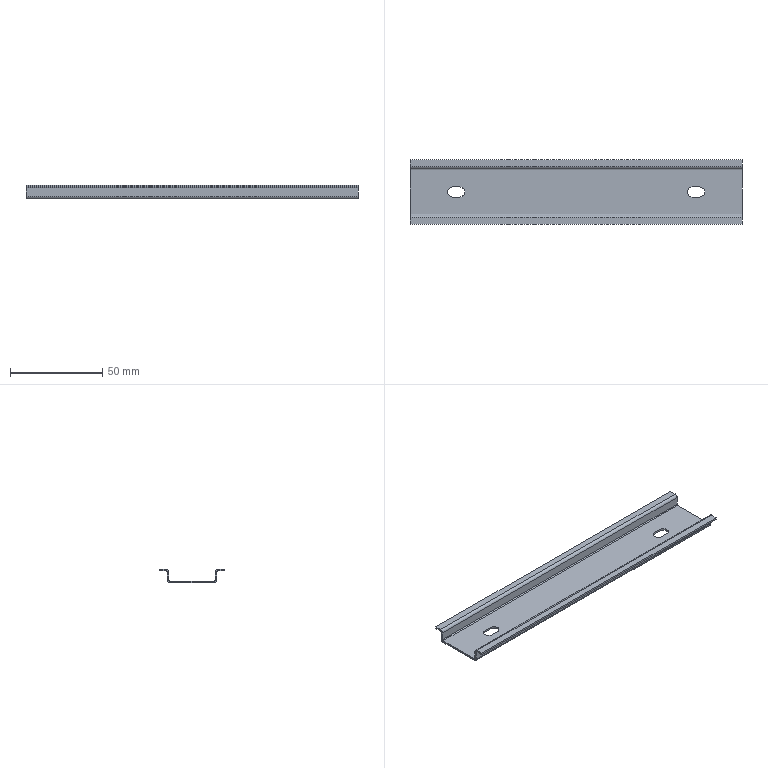Part | SolidWorks | features BaseBody 1 | 1 solid | 48 faces | box 180 x 35 x 7.5 mm | volume 8239 mm3 | plane 34 | cylinder 14 | commonest cylinder face diameters 5.5 x6 1 x4 3 x4
STEP:
#1=CARTESIAN_POINT('',(-67.,-2.75,0.));
#2=VERTEX_POINT('',#1);
#3=CARTESIAN_POINT('',(-63.,-2.75,0.));
#4=VERTEX_POINT('',#3);
#5=CARTESIAN_POINT('',(-67.,-2.75,0.));
#6=DIRECTION('',(1.,0.,0.));
#7=VECTOR('',#6,1000.);
#8=LINE('',#5,#7);
#9=EDGE_CURVE('',#2,#4,#8,.T.);
#10=ORIENTED_EDGE('',*,*,#9,.T.);
#11=CARTESIAN_POINT('',(-63.,-2.75,-1.));
#12=VERTEX_POINT('',#11);
#13=CARTESIAN_POINT('',(-63.,-2.75,-1.));
#14=DIRECTION('',(0.,0.,1.));
#15=VECTOR('',#14,1000.);
#16=LINE('',#13,#15);
#17=EDGE_CURVE('',#12,#4,#16,.T.);
#18=ORIENTED_EDGE('',*,*,#17,.F.);
#19=CARTESIAN_POINT('',(-67.,-2.75,-1.));
#20=VERTEX_POINT('',#19);
#21=CARTESIAN_POINT('',(-67.,-2.75,-1.));
#22=DIRECTION('',(1.,0.,0.));
#23=VECTOR('',#22,1000.);
#24=LINE('',#21,#23);
#25=EDGE_CURVE('',#20,#12,#24,.T.);
#26=ORIENTED_EDGE('',*,*,#25,.F.);
#27=CARTESIAN_POINT('',(-67.,-2.75,-1.));
#28=DIRECTION('',(0.,0.,1.));
#29=VECTOR('',#28,1000.);
#30=LINE('',#27,#29);
#31=EDGE_CURVE('',#20,#2,#30,.T.);
#32=ORIENTED_EDGE('',*,*,#31,.T.);
#33=EDGE_LOOP('',(#10,#18,#26,#32));
#34=FACE_OUTER_BOUND('',#33,.T.);
#35=CARTESIAN_POINT('',(-67.,-2.75,-1.));
#36=DIRECTION('',(0.,-1.,0.));
#37=DIRECTION('',(-1.,0.,0.));
#38=AXIS2_PLACEMENT_3D('',#35,#36,#37);
#39=PLANE('',#38);
#40=ADVANCED_FACE('',(#34),#39,.F.);
#41=CARTESIAN_POINT('',(-60.25,0.,-1.));
#42=VERTEX_POINT('',#41);
#43=CARTESIAN_POINT('',(-60.25,0.,0.));
#44=VERTEX_POINT('',#43);
#45=CARTESIAN_POINT('',(-60.25,0.,-1.));
#46=DIRECTION('',(0.,0.,1.));
#47=VECTOR('',#46,1000.);
#48=LINE('',#45,#47);
#49=EDGE_CURVE('',#42,#44,#48,.T.);
#50=ORIENTED_EDGE('',*,*,#49,.F.);
#51=CARTESIAN_POINT('',(-63.,0.,-1.));
#52=DIRECTION('',(0.,0.,1.));
#53=DIRECTION('',(1.,0.,0.));
#54=AXIS2_PLACEMENT_3D('',#51,#52,#53);
#55=CIRCLE('',#54,2.75);
#56=EDGE_CURVE('',#12,#42,#55,.T.);
#57=ORIENTED_EDGE('',*,*,#56,.F.);
#58=ORIENTED_EDGE('',*,*,#17,.T.);
#59=CARTESIAN_POINT('',(-63.,0.,0.));
#60=DIRECTION('',(0.,0.,1.));
#61=DIRECTION('',(1.,0.,0.));
#62=AXIS2_PLACEMENT_3D('',#59,#60,#61);
#63=CIRCLE('',#62,2.75);
#64=EDGE_CURVE('',#4,#44,#63,.T.);
#65=ORIENTED_EDGE('',*,*,#64,.T.);
#66=EDGE_LOOP('',(#50,#57,#58,#65));
#67=FACE_OUTER_BOUND('',#66,.T.);
#68=CARTESIAN_POINT('',(-63.,0.,-1.));
#69=DIRECTION('',(0.,0.,1.));
#70=DIRECTION('',(1.,0.,0.));
#71=AXIS2_PLACEMENT_3D('',#68,#69,#70);
#72=CYLINDRICAL_SURFACE('',#71,2.75);
#73=ADVANCED_FACE('',(#67),#72,.F.);
#74=CARTESIAN_POINT('',(-63.,2.75,0.));
#75=VERTEX_POINT('',#74);
#76=CARTESIAN_POINT('',(-67.,2.75,0.));
#77=VERTEX_POINT('',#76);
#78=CARTESIAN_POINT('',(-67.,2.75,0.));
#79=DIRECTION('',(-1.,0.,0.));
#80=VECTOR('',#79,1000.);
#81=LINE('',#78,#80);
#82=EDGE_CURVE('',#75,#77,#81,.T.);
#83=ORIENTED_EDGE('',*,*,#82,.T.);
#84=CARTESIAN_POINT('',(-67.,2.75,-1.));
#85=VERTEX_POINT('',#84);
#86=CARTESIAN_POINT('',(-67.,2.75,-1.));
#87=DIRECTION('',(0.,0.,1.));
#88=VECTOR('',#87,1000.);
#89=LINE('',#86,#88);
#90=EDGE_CURVE('',#85,#77,#89,.T.);
#91=ORIENTED_EDGE('',*,*,#90,.F.);
#92=CARTESIAN_POINT('',(-63.,2.75,-1.));
#93=VERTEX_POINT('',#92);
#94=CARTESIAN_POINT('',(-67.,2.75,-1.));
#95=DIRECTION('',(-1.,0.,0.));
#96=VECTOR('',#95,1000.);
#97=LINE('',#94,#96);
#98=EDGE_CURVE('',#93,#85,#97,.T.);
#99=ORIENTED_EDGE('',*,*,#98,.F.);
#100=CARTESIAN_POINT('',(-63.,2.75,-1.));
#101=DIRECTION('',(0.,0.,1.));
#102=VECTOR('',#101,1000.);
#103=LINE('',#100,#102);
#104=EDGE_CURVE('',#93,#75,#103,.T.);
#105=ORIENTED_EDGE('',*,*,#104,.T.);
#106=EDGE_LOOP('',(#83,#91,#99,#105));
#107=FACE_OUTER_BOUND('',#106,.T.);
#108=CARTESIAN_POINT('',(-67.,2.75,-1.));
#109=DIRECTION('',(0.,1.,0.));
#110=DIRECTION('',(1.,0.,0.));
#111=AXIS2_PLACEMENT_3D('',#108,#109,#110);
#112=PLANE('',#111);
#113=ADVANCED_FACE('',(#107),#112,.F.);
#114=CARTESIAN_POINT('',(-67.,0.,0.));
#115=DIRECTION('',(0.,0.,1.));
#116=DIRECTION('',(1.,0.,0.));
#117=AXIS2_PLACEMENT_3D('',#114,#115,#116);
#118=CIRCLE('',#117,2.75);
#119=EDGE_CURVE('',#77,#2,#118,.T.);
#120=ORIENTED_EDGE('',*,*,#119,.T.);
#121=ORIENTED_EDGE('',*,*,#31,.F.);
#122=CARTESIAN_POINT('',(-67.,0.,-1.));
#123=DIRECTION('',(0.,0.,1.));
#124=DIRECTION('',(1.,0.,0.));
#125=AXIS2_PLACEMENT_3D('',#122,#123,#124);
#126=CIRCLE('',#125,2.75);
#127=EDGE_CURVE('',#85,#20,#126,.T.);
#128=ORIENTED_EDGE('',*,*,#127,.F.);
#129=ORIENTED_EDGE('',*,*,#90,.T.);
#130=EDGE_LOOP('',(#120,#121,#128,#129));
#131=FACE_OUTER_BOUND('',#130,.T.);
#132=CARTESIAN_POINT('',(-67.,0.,-1.));
#133=DIRECTION('',(0.,0.,1.));
#134=DIRECTION('',(1.,0.,0.));
#135=AXIS2_PLACEMENT_3D('',#132,#133,#134);
#136=CYLINDRICAL_SURFACE('',#135,2.75);
#137=ADVANCED_FACE('',(#131),#136,.F.);
#138=CARTESIAN_POINT('',(67.,2.75,0.));
#139=VERTEX_POINT('',#138);
#140=CARTESIAN_POINT('',(63.,2.75,0.));
#141=VERTEX_POINT('',#140);
#142=CARTESIAN_POINT('',(67.,2.75,0.));
#143=DIRECTION('',(-1.,0.,0.));
#144=VECTOR('',#143,1000.);
#145=LINE('',#142,#144);
#146=EDGE_CURVE('',#139,#141,#145,.T.);
#147=ORIENTED_EDGE('',*,*,#146,.T.);
#148=CARTESIAN_POINT('',(63.,2.75,-1.));
#149=VERTEX_POINT('',#148);
#150=CARTESIAN_POINT('',(63.,2.75,-1.));
#151=DIRECTION('',(0.,0.,1.));
#152=VECTOR('',#151,1000.);
#153=LINE('',#150,#152);
#154=EDGE_CURVE('',#149,#141,#153,.T.);
#155=ORIENTED_EDGE('',*,*,#154,.F.);
#156=CARTESIAN_POINT('',(67.,2.75,-1.));
#157=VERTEX_POINT('',#156);
#158=CARTESIAN_POINT('',(67.,2.75,-1.));
#159=DIRECTION('',(-1.,0.,0.));
#160=VECTOR('',#159,1000.);
#161=LINE('',#158,#160);
#162=EDGE_CURVE('',#157,#149,#161,.T.);
#163=ORIENTED_EDGE('',*,*,#162,.F.);
#164=CARTESIAN_POINT('',(67.,2.75,-1.));
#165=DIRECTION('',(0.,0.,1.));
#166=VECTOR('',#165,1000.);
#167=LINE('',#164,#166);
#168=EDGE_CURVE('',#157,#139,#167,.T.);
#169=ORIENTED_EDGE('',*,*,#168,.T.);
#170=EDGE_LOOP('',(#147,#155,#163,#169));
#171=FACE_OUTER_BOUND('',#170,.T.);
#172=CARTESIAN_POINT('',(67.,2.75,-1.));
#173=DIRECTION('',(0.,1.,0.));
#174=DIRECTION('',(1.,0.,0.));
#175=AXIS2_PLACEMENT_3D('',#172,#173,#174);
#176=PLANE('',#175);
#177=ADVANCED_FACE('',(#171),#176,.F.);
#178=CARTESIAN_POINT('',(63.,-2.75,0.));
#179=VERTEX_POINT('',#178);
#180=CARTESIAN_POINT('',(63.,0.,0.));
#181=DIRECTION('',(0.,0.,1.));
#182=DIRECTION('',(-1.,0.,0.));
#183=AXIS2_PLACEMENT_3D('',#180,#181,#182);
#184=CIRCLE('',#183,2.75);
#185=EDGE_CURVE('',#141,#179,#184,.T.);
#186=ORIENTED_EDGE('',*,*,#185,.T.);
#187=CARTESIAN_POINT('',(63.,-2.75,-1.));
#188=VERTEX_POINT('',#187);
#189=CARTESIAN_POINT('',(63.,-2.75,-1.));
#190=DIRECTION('',(0.,0.,1.));
#191=VECTOR('',#190,1000.);
#192=LINE('',#189,#191);
#193=EDGE_CURVE('',#188,#179,#192,.T.);
#194=ORIENTED_EDGE('',*,*,#193,.F.);
#195=CARTESIAN_POINT('',(63.,0.,-1.));
#196=DIRECTION('',(0.,0.,1.));
#197=DIRECTION('',(-1.,0.,0.));
#198=AXIS2_PLACEMENT_3D('',#195,#196,#197);
#199=CIRCLE('',#198,2.75);
#200=EDGE_CURVE('',#149,#188,#199,.T.);
#201=ORIENTED_EDGE('',*,*,#200,.F.);
#202=ORIENTED_EDGE('',*,*,#154,.T.);
#203=EDGE_LOOP('',(#186,#194,#201,#202));
#204=FACE_OUTER_BOUND('',#203,.T.);
#205=CARTESIAN_POINT('',(63.,0.,-1.));
#206=DIRECTION('',(0.,0.,1.));
#207=DIRECTION('',(1.,0.,0.));
#208=AXIS2_PLACEMENT_3D('',#205,#206,#207);
#209=CYLINDRICAL_SURFACE('',#208,2.75);
#210=ADVANCED_FACE('',(#204),#209,.F.);
#211=CARTESIAN_POINT('',(67.,-2.75,0.));
#212=VERTEX_POINT('',#211);
#213=CARTESIAN_POINT('',(67.,-2.75,0.));
#214=DIRECTION('',(1.,0.,0.));
#215=VECTOR('',#214,1000.);
#216=LINE('',#213,#215);
#217=EDGE_CURVE('',#179,#212,#216,.T.);
#218=ORIENTED_EDGE('',*,*,#217,.T.);
#219=CARTESIAN_POINT('',(67.,-2.75,-1.));
#220=VERTEX_POINT('',#219);
#221=CARTESIAN_POINT('',(67.,-2.75,-1.));
#222=DIRECTION('',(0.,0.,1.));
#223=VECTOR('',#222,1000.);
#224=LINE('',#221,#223);
#225=EDGE_CURVE('',#220,#212,#224,.T.);
#226=ORIENTED_EDGE('',*,*,#225,.F.);
#227=CARTESIAN_POINT('',(67.,-2.75,-1.));
#228=DIRECTION('',(1.,0.,0.));
#229=VECTOR('',#228,1000.);
#230=LINE('',#227,#229);
#231=EDGE_CURVE('',#188,#220,#230,.T.);
#232=ORIENTED_EDGE('',*,*,#231,.F.);
#233=ORIENTED_EDGE('',*,*,#193,.T.);
#234=EDGE_LOOP('',(#218,#226,#232,#233));
#235=FACE_OUTER_BOUND('',#234,.T.);
#236=CARTESIAN_POINT('',(67.,-2.75,-1.));
#237=DIRECTION('',(0.,-1.,0.));
#238=DIRECTION('',(0.,0.,-1.));
#239=AXIS2_PLACEMENT_3D('',#236,#237,#238);
#240=PLANE('',#239);
#241=ADVANCED_FACE('',(#235),#240,.F.);
#242=CARTESIAN_POINT('',(69.75,0.,-1.));
#243=VERTEX_POINT('',#242);
#244=CARTESIAN_POINT('',(69.75,0.,0.));
#245=VERTEX_POINT('',#244);
#246=CARTESIAN_POINT('',(69.75,0.,-1.));
#247=DIRECTION('',(0.,0.,1.));
#248=VECTOR('',#247,1000.);
#249=LINE('',#246,#248);
#250=EDGE_CURVE('',#243,#245,#249,.T.);
#251=ORIENTED_EDGE('',*,*,#250,.F.);
#252=CARTESIAN_POINT('',(67.,0.,-1.));
#253=DIRECTION('',(0.,0.,1.));
#254=DIRECTION('',(-1.,0.,0.));
#255=AXIS2_PLACEMENT_3D('',#252,#253,#254);
#256=CIRCLE('',#255,2.75);
#257=EDGE_CURVE('',#220,#243,#256,.T.);
#258=ORIENTED_EDGE('',*,*,#257,.F.);
#259=ORIENTED_EDGE('',*,*,#225,.T.);
#260=CARTESIAN_POINT('',(67.,0.,0.));
#261=DIRECTION('',(0.,0.,1.));
#262=DIRECTION('',(-1.,0.,0.));
#263=AXIS2_PLACEMENT_3D('',#260,#261,#262);
#264=CIRCLE('',#263,2.75);
#265=EDGE_CURVE('',#212,#245,#264,.T.);
#266=ORIENTED_EDGE('',*,*,#265,.T.);
#267=EDGE_LOOP('',(#251,#258,#259,#266));
#268=FACE_OUTER_BOUND('',#267,.T.);
#269=CARTESIAN_POINT('',(67.,0.,-1.));
#270=DIRECTION('',(0.,0.,1.));
#271=DIRECTION('',(1.,0.,0.));
#272=AXIS2_PLACEMENT_3D('',#269,#270,#271);
#273=CYLINDRICAL_SURFACE('',#272,2.75);
#274=ADVANCED_FACE('',(#268),#273,.F.);
#275=CARTESIAN_POINT('',(-90.,-17.5,5.5));
#276=VERTEX_POINT('',#275);
#277=CARTESIAN_POINT('',(90.,-17.5,5.5));
#278=VERTEX_POINT('',#277);
#279=CARTESIAN_POINT('',(90.,-17.5,5.5));
#280=DIRECTION('',(1.,0.,0.));
#281=VECTOR('',#280,1000.);
#282=LINE('',#279,#281);
#283=EDGE_CURVE('',#276,#278,#282,.T.);
#284=ORIENTED_EDGE('',*,*,#283,.T.);
#285=CARTESIAN_POINT('',(90.,-17.5,6.5));
#286=VERTEX_POINT('',#285);
#287=CARTESIAN_POINT('',(90.,-17.5,6.5));
#288=DIRECTION('',(0.,0.,-1.));
#289=VECTOR('',#288,1000.);
#290=LINE('',#287,#289);
#291=EDGE_CURVE('',#286,#278,#290,.T.);
#292=ORIENTED_EDGE('',*,*,#291,.F.);
#293=CARTESIAN_POINT('',(-90.,-17.5,6.5));
#294=VERTEX_POINT('',#293);
#295=CARTESIAN_POINT('',(0.,-17.5,6.5));
#296=DIRECTION('',(1.,0.,0.));
#297=VECTOR('',#296,1000.);
#298=LINE('',#295,#297);
#299=EDGE_CURVE('',#294,#286,#298,.T.);
#300=ORIENTED_EDGE('',*,*,#299,.F.);
#301=CARTESIAN_POINT('',(-90.,-17.5,6.5));
#302=DIRECTION('',(0.,0.,-1.));
#303=VECTOR('',#302,1000.);
#304=LINE('',#301,#303);
#305=EDGE_CURVE('',#294,#276,#304,.T.);
#306=ORIENTED_EDGE('',*,*,#305,.T.);
#307=EDGE_LOOP('',(#284,#292,#300,#306));
#308=FACE_OUTER_BOUND('',#307,.T.);
#309=CARTESIAN_POINT('',(90.,-17.5,6.5));
#310=DIRECTION('',(0.,1.,0.));
#311=DIRECTION('',(0.,0.,-1.));
#312=AXIS2_PLACEMENT_3D('',#309,#310,#311);
#313=PLANE('',#312);
#314=ADVANCED_FACE('',(#308),#313,.F.);
#315=CARTESIAN_POINT('',(-90.,-14.,5.5));
#316=VERTEX_POINT('',#315);
#317=CARTESIAN_POINT('',(-90.,-17.5,5.5));
#318=DIRECTION('',(0.,-1.,0.));
#319=VECTOR('',#318,1000.);
#320=LINE('',#317,#319);
#321=EDGE_CURVE('',#316,#276,#320,.T.);
#322=ORIENTED_EDGE('',*,*,#321,.F.);
#323=CARTESIAN_POINT('',(90.,-14.,5.5));
#324=VERTEX_POINT('',#323);
#325=CARTESIAN_POINT('',(90.,-14.,5.5));
#326=DIRECTION('',(-1.,0.,0.));
#327=VECTOR('',#326,1000.);
#328=LINE('',#325,#327);
#329=EDGE_CURVE('',#324,#316,#328,.T.);
#330=ORIENTED_EDGE('',*,*,#329,.F.);
#331=CARTESIAN_POINT('',(90.,-13.5,5.5));
#332=DIRECTION('',(0.,1.,0.));
#333=VECTOR('',#332,1000.);
#334=LINE('',#331,#333);
#335=EDGE_CURVE('',#278,#324,#334,.T.);
#336=ORIENTED_EDGE('',*,*,#335,.F.);
#337=ORIENTED_EDGE('',*,*,#283,.F.);
#338=EDGE_LOOP('',(#322,#330,#336,#337));
#339=FACE_OUTER_BOUND('',#338,.T.);
#340=CARTESIAN_POINT('',(0.,0.,5.5));
#341=DIRECTION('',(0.,0.,-1.));
#342=DIRECTION('',(-1.,0.,0.));
#343=AXIS2_PLACEMENT_3D('',#340,#341,#342);
#344=PLANE('',#343);
#345=ADVANCED_FACE('',(#339),#344,.T.);
#346=CARTESIAN_POINT('',(-90.,-14.,6.5));
#347=VERTEX_POINT('',#346);
#348=CARTESIAN_POINT('',(90.,-14.,6.5));
#349=VERTEX_POINT('',#348);
#350=CARTESIAN_POINT('',(90.,-14.,6.5));
#351=DIRECTION('',(1.,0.,0.));
#352=VECTOR('',#351,1000.);
#353=LINE('',#350,#352);
#354=EDGE_CURVE('',#347,#349,#353,.T.);
#355=ORIENTED_EDGE('',*,*,#354,.F.);
#356=CARTESIAN_POINT('',(-90.,0.,6.5));
#357=DIRECTION('',(0.,-1.,0.));
#358=VECTOR('',#357,1000.);
#359=LINE('',#356,#358);
#360=EDGE_CURVE('',#347,#294,#359,.T.);
#361=ORIENTED_EDGE('',*,*,#360,.T.);
#362=ORIENTED_EDGE('',*,*,#299,.T.);
#363=CARTESIAN_POINT('',(90.,0.,6.5));
#364=DIRECTION('',(0.,1.,0.));
#365=VECTOR('',#364,1000.);
#366=LINE('',#363,#365);
#367=EDGE_CURVE('',#286,#349,#366,.T.);
#368=ORIENTED_EDGE('',*,*,#367,.T.);
#369=EDGE_LOOP('',(#355,#361,#362,#368));
#370=FACE_OUTER_BOUND('',#369,.T.);
#371=CARTESIAN_POINT('',(0.,0.,6.5));
#372=DIRECTION('',(0.,0.,-1.));
#373=DIRECTION('',(-1.,0.,0.));
#374=AXIS2_PLACEMENT_3D('',#371,#372,#373);
#375=PLANE('',#374);
#376=ADVANCED_FACE('',(#370),#375,.F.);
#377=CARTESIAN_POINT('',(-90.,-14.,5.5));
#378=DIRECTION('',(0.,0.,1.));
#379=VECTOR('',#378,1000.);
#380=LINE('',#377,#379);
#381=EDGE_CURVE('',#316,#347,#380,.T.);
#382=ORIENTED_EDGE('',*,*,#381,.F.);
#383=ORIENTED_EDGE('',*,*,#321,.T.);
#384=ORIENTED_EDGE('',*,*,#305,.F.);
#385=ORIENTED_EDGE('',*,*,#360,.F.);
#386=EDGE_LOOP('',(#382,#383,#384,#385));
#387=FACE_OUTER_BOUND('',#386,.T.);
#388=CARTESIAN_POINT('',(-90.,-17.5,6.5));
#389=DIRECTION('',(1.,0.,0.));
#390=DIRECTION('',(0.,0.,-1.));
#391=AXIS2_PLACEMENT_3D('',#388,#389,#390);
#392=PLANE('',#391);
#393=ADVANCED_FACE('',(#387),#392,.F.);
#394=CARTESIAN_POINT('',(90.,-14.,6.5));
#395=DIRECTION('',(0.,0.,1.));
#396=VECTOR('',#395,1000.);
#397=LINE('',#394,#396);
#398=EDGE_CURVE('',#324,#349,#397,.T.);
#399=ORIENTED_EDGE('',*,*,#398,.T.);
#400=ORIENTED_EDGE('',*,*,#367,.F.);
#401=ORIENTED_EDGE('',*,*,#291,.T.);
#402=ORIENTED_EDGE('',*,*,#335,.T.);
#403=EDGE_LOOP('',(#399,#400,#401,#402));
#404=FACE_OUTER_BOUND('',#403,.T.);
#405=CARTESIAN_POINT('',(90.,-13.5,6.5));
#406=DIRECTION('',(-1.,0.,0.));
#407=DIRECTION('',(0.,1.,0.));
#408=AXIS2_PLACEMENT_3D('',#405,#406,#407);
#409=PLANE('',#408);
#410=ADVANCED_FACE('',(#404),#409,.F.);
#411=CARTESIAN_POINT('',(-90.,-13.5,5.));
#412=VERTEX_POINT('',#411);
#413=CARTESIAN_POINT('',(90.,-13.5,5.));
#414=VERTEX_POINT('',#413);
#415=CARTESIAN_POINT('',(-90.,-13.5,5.));
#416=DIRECTION('',(1.,0.,0.));
#417=VECTOR('',#416,1000.);
#418=LINE('',#415,#417);
#419=EDGE_CURVE('',#412,#414,#418,.T.);
#420=ORIENTED_EDGE('',*,*,#419,.T.);
#421=CARTESIAN_POINT('',(90.,-14.,5.));
#422=DIRECTION('',(1.,0.,0.));
#423=DIRECTION('',(0.,0.,1.));
#424=AXIS2_PLACEMENT_3D('',#421,#422,#423);
#425=CIRCLE('',#424,0.5);
#426=EDGE_CURVE('',#414,#324,#425,.T.);
#427=ORIENTED_EDGE('',*,*,#426,.T.);
#428=ORIENTED_EDGE('',*,*,#329,.T.);
#429=CARTESIAN_POINT('',(-90.,-14.,5.));
#430=DIRECTION('',(-1.,0.,0.));
#431=DIRECTION('',(0.,0.,1.));
#432=AXIS2_PLACEMENT_3D('',#429,#430,#431);
#433=CIRCLE('',#432,0.5);
#434=EDGE_CURVE('',#316,#412,#433,.T.);
#435=ORIENTED_EDGE('',*,*,#434,.T.);
#436=EDGE_LOOP('',(#420,#427,#428,#435));
#437=FACE_OUTER_BOUND('',#436,.T.);
#438=CARTESIAN_POINT('',(-90.,-14.,5.));
#439=DIRECTION('',(-1.,0.,0.));
#440=DIRECTION('',(0.,0.,1.));
#441=AXIS2_PLACEMENT_3D('',#438,#439,#440);
#442=CYLINDRICAL_SURFACE('',#441,0.5);
#443=ADVANCED_FACE('',(#437),#442,.F.);
#444=CARTESIAN_POINT('',(-90.,-12.5,5.));
#445=VERTEX_POINT('',#444);
#446=CARTESIAN_POINT('',(90.,-12.5,5.));
#447=VERTEX_POINT('',#446);
#448=CARTESIAN_POINT('',(-90.,-12.5,5.));
#449=DIRECTION('',(1.,0.,0.));
#450=VECTOR('',#449,1000.);
#451=LINE('',#448,#450);
#452=EDGE_CURVE('',#445,#447,#451,.T.);
#453=ORIENTED_EDGE('',*,*,#452,.F.);
#454=CARTESIAN_POINT('',(-90.,-14.,5.));
#455=DIRECTION('',(-1.,0.,0.));
#456=DIRECTION('',(0.,0.,1.));
#457=AXIS2_PLACEMENT_3D('',#454,#455,#456);
#458=CIRCLE('',#457,1.5);
#459=EDGE_CURVE('',#347,#445,#458,.T.);
#460=ORIENTED_EDGE('',*,*,#459,.F.);
#461=ORIENTED_EDGE('',*,*,#354,.T.);
#462=CARTESIAN_POINT('',(90.,-14.,5.));
#463=DIRECTION('',(1.,0.,0.));
#464=DIRECTION('',(0.,0.,1.));
#465=AXIS2_PLACEMENT_3D('',#462,#463,#464);
#466=CIRCLE('',#465,1.5);
#467=EDGE_CURVE('',#447,#349,#466,.T.);
#468=ORIENTED_EDGE('',*,*,#467,.F.);
#469=EDGE_LOOP('',(#453,#460,#461,#468));
#470=FACE_OUTER_BOUND('',#469,.T.);
#471=CARTESIAN_POINT('',(-90.,-14.,5.));
#472=DIRECTION('',(-1.,0.,0.));
#473=DIRECTION('',(0.,0.,1.));
#474=AXIS2_PLACEMENT_3D('',#471,#472,#473);
#475=CYLINDRICAL_SURFACE('',#474,1.5);
#476=ADVANCED_FACE('',(#470),#475,.T.);
#477=ORIENTED_EDGE('',*,*,#434,.F.);
#478=ORIENTED_EDGE('',*,*,#381,.T.);
#479=ORIENTED_EDGE('',*,*,#459,.T.);
#480=CARTESIAN_POINT('',(-90.,-13.5,5.));
#481=DIRECTION('',(0.,1.,0.));
#482=VECTOR('',#481,1000.);
#483=LINE('',#480,#482);
#484=EDGE_CURVE('',#412,#445,#483,.T.);
#485=ORIENTED_EDGE('',*,*,#484,.F.);
#486=EDGE_LOOP('',(#477,#478,#479,#485));
#487=FACE_OUTER_BOUND('',#486,.T.);
#488=CARTESIAN_POINT('',(-90.,-14.,5.));
#489=DIRECTION('',(1.,0.,0.));
#490=DIRECTION('',(0.,1.,0.));
#491=AXIS2_PLACEMENT_3D('',#488,#489,#490);
#492=PLANE('',#491);
#493=ADVANCED_FACE('',(#487),#492,.F.);
#494=ORIENTED_EDGE('',*,*,#398,.F.);
#495=ORIENTED_EDGE('',*,*,#426,.F.);
#496=CARTESIAN_POINT('',(90.,-13.5,5.));
#497=DIRECTION('',(0.,1.,0.));
#498=VECTOR('',#497,1000.);
#499=LINE('',#496,#498);
#500=EDGE_CURVE('',#414,#447,#499,.T.);
#501=ORIENTED_EDGE('',*,*,#500,.T.);
#502=ORIENTED_EDGE('',*,*,#467,.T.);
#503=EDGE_LOOP('',(#494,#495,#501,#502));
#504=FACE_OUTER_BOUND('',#503,.T.);
#505=CARTESIAN_POINT('',(90.,-14.,5.));
#506=DIRECTION('',(1.,0.,0.));
#507=DIRECTION('',(0.,1.,0.));
#508=AXIS2_PLACEMENT_3D('',#505,#506,#507);
#509=PLANE('',#508);
#510=ADVANCED_FACE('',(#504),#509,.T.);
#511=CARTESIAN_POINT('',(90.,17.5,5.5));
#512=VERTEX_POINT('',#511);
#513=CARTESIAN_POINT('',(-90.,17.5,5.5));
#514=VERTEX_POINT('',#513);
#515=CARTESIAN_POINT('',(-90.,17.5,5.5));
#516=DIRECTION('',(-1.,0.,0.));
#517=VECTOR('',#516,1000.);
#518=LINE('',#515,#517);
#519=EDGE_CURVE('',#512,#514,#518,.T.);
#520=ORIENTED_EDGE('',*,*,#519,.T.);
#521=CARTESIAN_POINT('',(-90.,17.5,6.5));
#522=VERTEX_POINT('',#521);
#523=CARTESIAN_POINT('',(-90.,17.5,6.5));
#524=DIRECTION('',(0.,0.,-1.));
#525=VECTOR('',#524,1000.);
#526=LINE('',#523,#525);
#527=EDGE_CURVE('',#522,#514,#526,.T.);
#528=ORIENTED_EDGE('',*,*,#527,.F.);
#529=CARTESIAN_POINT('',(90.,17.5,6.5));
#530=VERTEX_POINT('',#529);
#531=CARTESIAN_POINT('',(0.,17.5,6.5));
#532=DIRECTION('',(-1.,0.,0.));
#533=VECTOR('',#532,1000.);
#534=LINE('',#531,#533);
#535=EDGE_CURVE('',#530,#522,#534,.T.);
#536=ORIENTED_EDGE('',*,*,#535,.F.);
#537=CARTESIAN_POINT('',(90.,17.5,6.5));
#538=DIRECTION('',(0.,0.,-1.));
#539=VECTOR('',#538,1000.);
#540=LINE('',#537,#539);
#541=EDGE_CURVE('',#530,#512,#540,.T.);
#542=ORIENTED_EDGE('',*,*,#541,.T.);
#543=EDGE_LOOP('',(#520,#528,#536,#542));
#544=FACE_OUTER_BOUND('',#543,.T.);
#545=CARTESIAN_POINT('',(-90.,17.5,6.5));
#546=DIRECTION('',(0.,-1.,0.));
#547=DIRECTION('',(0.,0.,-1.));
#548=AXIS2_PLACEMENT_3D('',#545,#546,#547);
#549=PLANE('',#548);
#550=ADVANCED_FACE('',(#544),#549,.F.);
#551=CARTESIAN_POINT('',(90.,14.,5.5));
#552=VERTEX_POINT('',#551);
#553=CARTESIAN_POINT('',(90.,17.5,5.5));
#554=DIRECTION('',(0.,1.,0.));
#555=VECTOR('',#554,1000.);
#556=LINE('',#553,#555);
#557=EDGE_CURVE('',#552,#512,#556,.T.);
#558=ORIENTED_EDGE('',*,*,#557,.F.);
#559=CARTESIAN_POINT('',(-90.,14.,5.5));
#560=VERTEX_POINT('',#559);
#561=CARTESIAN_POINT('',(-90.,14.,5.5));
#562=DIRECTION('',(1.,0.,0.));
#563=VECTOR('',#562,1000.);
#564=LINE('',#561,#563);
#565=EDGE_CURVE('',#560,#552,#564,.T.);
#566=ORIENTED_EDGE('',*,*,#565,.F.);
#567=CARTESIAN_POINT('',(-90.,13.5,5.5));
#568=DIRECTION('',(0.,-1.,0.));
#569=VECTOR('',#568,1000.);
#570=LINE('',#567,#569);
#571=EDGE_CURVE('',#514,#560,#570,.T.);
#572=ORIENTED_EDGE('',*,*,#571,.F.);
#573=ORIENTED_EDGE('',*,*,#519,.F.);
#574=EDGE_LOOP('',(#558,#566,#572,#573));
#575=FACE_OUTER_BOUND('',#574,.T.);
#576=CARTESIAN_POINT('',(0.,0.,5.5));
#577=DIRECTION('',(0.,0.,-1.));
#578=DIRECTION('',(0.,-1.,0.));
#579=AXIS2_PLACEMENT_3D('',#576,#577,#578);
#580=PLANE('',#579);
#581=ADVANCED_FACE('',(#575),#580,.T.);
#582=CARTESIAN_POINT('',(90.,14.,6.5));
#583=VERTEX_POINT('',#582);
#584=CARTESIAN_POINT('',(-90.,14.,6.5));
#585=VERTEX_POINT('',#584);
#586=CARTESIAN_POINT('',(-90.,14.,6.5));
#587=DIRECTION('',(-1.,0.,0.));
#588=VECTOR('',#587,1000.);
#589=LINE('',#586,#588);
#590=EDGE_CURVE('',#583,#585,#589,.T.);
#591=ORIENTED_EDGE('',*,*,#590,.F.);
#592=CARTESIAN_POINT('',(90.,0.,6.5));
#593=DIRECTION('',(0.,1.,0.));
#594=VECTOR('',#593,1000.);
#595=LINE('',#592,#594);
#596=EDGE_CURVE('',#583,#530,#595,.T.);
#597=ORIENTED_EDGE('',*,*,#596,.T.);
#598=ORIENTED_EDGE('',*,*,#535,.T.);
#599=CARTESIAN_POINT('',(-90.,0.,6.5));
#600=DIRECTION('',(0.,-1.,0.));
#601=VECTOR('',#600,1000.);
#602=LINE('',#599,#601);
#603=EDGE_CURVE('',#522,#585,#602,.T.);
#604=ORIENTED_EDGE('',*,*,#603,.T.);
#605=EDGE_LOOP('',(#591,#597,#598,#604));
#606=FACE_OUTER_BOUND('',#605,.T.);
#607=CARTESIAN_POINT('',(0.,0.,6.5));
#608=DIRECTION('',(0.,0.,-1.));
#609=DIRECTION('',(0.,-1.,0.));
#610=AXIS2_PLACEMENT_3D('',#607,#608,#609);
#611=PLANE('',#610);
#612=ADVANCED_FACE('',(#606),#611,.F.);
#613=CARTESIAN_POINT('',(90.,14.,5.5));
#614=DIRECTION('',(0.,0.,1.));
#615=VECTOR('',#614,1000.);
#616=LINE('',#613,#615);
#617=EDGE_CURVE('',#552,#583,#616,.T.);
#618=ORIENTED_EDGE('',*,*,#617,.F.);
#619=ORIENTED_EDGE('',*,*,#557,.T.);
#620=ORIENTED_EDGE('',*,*,#541,.F.);
#621=ORIENTED_EDGE('',*,*,#596,.F.);
#622=EDGE_LOOP('',(#618,#619,#620,#621));
#623=FACE_OUTER_BOUND('',#622,.T.);
#624=CARTESIAN_POINT('',(90.,17.5,6.5));
#625=DIRECTION('',(-1.,0.,0.));
#626=DIRECTION('',(0.,0.,1.));
#627=AXIS2_PLACEMENT_3D('',#624,#625,#626);
#628=PLANE('',#627);
#629=ADVANCED_FACE('',(#623),#628,.F.);
#630=CARTESIAN_POINT('',(-90.,14.,6.5));
#631=DIRECTION('',(0.,0.,1.));
#632=VECTOR('',#631,1000.);
#633=LINE('',#630,#632);
#634=EDGE_CURVE('',#560,#585,#633,.T.);
#635=ORIENTED_EDGE('',*,*,#634,.T.);
#636=ORIENTED_EDGE('',*,*,#603,.F.);
#637=ORIENTED_EDGE('',*,*,#527,.T.);
#638=ORIENTED_EDGE('',*,*,#571,.T.);
#639=EDGE_LOOP('',(#635,#636,#637,#638));
#640=FACE_OUTER_BOUND('',#639,.T.);
#641=CARTESIAN_POINT('',(-90.,13.5,6.5));
#642=DIRECTION('',(1.,0.,0.));
#643=DIRECTION('',(0.,1.,0.));
#644=AXIS2_PLACEMENT_3D('',#641,#642,#643);
#645=PLANE('',#644);
#646=ADVANCED_FACE('',(#640),#645,.F.);
#647=CARTESIAN_POINT('',(90.,13.5,5.));
#648=VERTEX_POINT('',#647);
#649=CARTESIAN_POINT('',(-90.,13.5,5.));
#650=VERTEX_POINT('',#649);
#651=CARTESIAN_POINT('',(90.,13.5,5.));
#652=DIRECTION('',(-1.,0.,0.));
#653=VECTOR('',#652,1000.);
#654=LINE('',#651,#653);
#655=EDGE_CURVE('',#648,#650,#654,.T.);
#656=ORIENTED_EDGE('',*,*,#655,.T.);
#657=CARTESIAN_POINT('',(-90.,14.,5.));
#658=DIRECTION('',(-1.,0.,0.));
#659=DIRECTION('',(0.,0.,-1.));
#660=AXIS2_PLACEMENT_3D('',#657,#658,#659);
#661=CIRCLE('',#660,0.5);
#662=EDGE_CURVE('',#650,#560,#661,.T.);
#663=ORIENTED_EDGE('',*,*,#662,.T.);
#664=ORIENTED_EDGE('',*,*,#565,.T.);
#665=CARTESIAN_POINT('',(90.,14.,5.));
#666=DIRECTION('',(1.,0.,0.));
#667=DIRECTION('',(0.,0.,-1.));
#668=AXIS2_PLACEMENT_3D('',#665,#666,#667);
#669=CIRCLE('',#668,0.5);
#670=EDGE_CURVE('',#552,#648,#669,.T.);
#671=ORIENTED_EDGE('',*,*,#670,.T.);
#672=EDGE_LOOP('',(#656,#663,#664,#671));
#673=FACE_OUTER_BOUND('',#672,.T.);
#674=CARTESIAN_POINT('',(90.,14.,5.));
#675=DIRECTION('',(1.,0.,0.));
#676=DIRECTION('',(0.,0.,1.));
#677=AXIS2_PLACEMENT_3D('',#674,#675,#676);
#678=CYLINDRICAL_SURFACE('',#677,0.5);
#679=ADVANCED_FACE('',(#673),#678,.F.);
#680=CARTESIAN_POINT('',(90.,12.5,5.));
#681=VERTEX_POINT('',#680);
#682=CARTESIAN_POINT('',(-90.,12.5,5.));
#683=VERTEX_POINT('',#682);
#684=CARTESIAN_POINT('',(90.,12.5,5.));
#685=DIRECTION('',(-1.,0.,0.));
#686=VECTOR('',#685,1000.);
#687=LINE('',#684,#686);
#688=EDGE_CURVE('',#681,#683,#687,.T.);
#689=ORIENTED_EDGE('',*,*,#688,.F.);
#690=CARTESIAN_POINT('',(90.,14.,5.));
#691=DIRECTION('',(1.,0.,0.));
#692=DIRECTION('',(0.,0.,-1.));
#693=AXIS2_PLACEMENT_3D('',#690,#691,#692);
#694=CIRCLE('',#693,1.5);
#695=EDGE_CURVE('',#583,#681,#694,.T.);
#696=ORIENTED_EDGE('',*,*,#695,.F.);
#697=ORIENTED_EDGE('',*,*,#590,.T.);
#698=CARTESIAN_POINT('',(-90.,14.,5.));
#699=DIRECTION('',(-1.,0.,0.));
#700=DIRECTION('',(0.,0.,-1.));
#701=AXIS2_PLACEMENT_3D('',#698,#699,#700);
#702=CIRCLE('',#701,1.5);
#703=EDGE_CURVE('',#683,#585,#702,.T.);
#704=ORIENTED_EDGE('',*,*,#703,.F.);
#705=EDGE_LOOP('',(#689,#696,#697,#704));
#706=FACE_OUTER_BOUND('',#705,.T.);
#707=CARTESIAN_POINT('',(90.,14.,5.));
#708=DIRECTION('',(1.,0.,0.));
#709=DIRECTION('',(0.,0.,1.));
#710=AXIS2_PLACEMENT_3D('',#707,#708,#709);
#711=CYLINDRICAL_SURFACE('',#710,1.5);
#712=ADVANCED_FACE('',(#706),#711,.T.);
#713=ORIENTED_EDGE('',*,*,#670,.F.);
#714=ORIENTED_EDGE('',*,*,#617,.T.);
#715=ORIENTED_EDGE('',*,*,#695,.T.);
#716=CARTESIAN_POINT('',(90.,13.5,5.));
#717=DIRECTION('',(0.,-1.,0.));
#718=VECTOR('',#717,1000.);
#719=LINE('',#716,#718);
#720=EDGE_CURVE('',#648,#681,#719,.T.);
#721=ORIENTED_EDGE('',*,*,#720,.F.);
#722=EDGE_LOOP('',(#713,#714,#715,#721));
#723=FACE_OUTER_BOUND('',#722,.T.);
#724=CARTESIAN_POINT('',(90.,14.,5.));
#725=DIRECTION('',(-1.,0.,0.));
#726=DIRECTION('',(0.,0.,1.));
#727=AXIS2_PLACEMENT_3D('',#724,#725,#726);
#728=PLANE('',#727);
#729=ADVANCED_FACE('',(#723),#728,.F.);
#730=ORIENTED_EDGE('',*,*,#634,.F.);
#731=ORIENTED_EDGE('',*,*,#662,.F.);
#732=CARTESIAN_POINT('',(-90.,13.5,5.));
#733=DIRECTION('',(0.,-1.,0.));
#734=VECTOR('',#733,1000.);
#735=LINE('',#732,#734);
#736=EDGE_CURVE('',#650,#683,#735,.T.);
#737=ORIENTED_EDGE('',*,*,#736,.T.);
#738=ORIENTED_EDGE('',*,*,#703,.T.);
#739=EDGE_LOOP('',(#730,#731,#737,#738));
#740=FACE_OUTER_BOUND('',#739,.T.);
#741=CARTESIAN_POINT('',(-90.,14.,5.));
#742=DIRECTION('',(-1.,0.,0.));
#743=DIRECTION('',(0.,0.,1.));
#744=AXIS2_PLACEMENT_3D('',#741,#742,#743);
#745=PLANE('',#744);
#746=ADVANCED_FACE('',(#740),#745,.T.);
#747=CARTESIAN_POINT('',(90.,-12.,0.));
#748=VERTEX_POINT('',#747);
#749=CARTESIAN_POINT('',(-90.,-12.,0.));
#750=VERTEX_POINT('',#749);
#751=CARTESIAN_POINT('',(90.,-12.,0.));
#752=DIRECTION('',(-1.,0.,0.));
#753=VECTOR('',#752,1000.);
#754=LINE('',#751,#753);
#755=EDGE_CURVE('',#748,#750,#754,.T.);
#756=ORIENTED_EDGE('',*,*,#755,.T.);
#757=CARTESIAN_POINT('',(-90.,-12.5,0.5));
#758=VERTEX_POINT('',#757);
#759=CARTESIAN_POINT('',(-90.,-12.,0.5));
#760=DIRECTION('',(-1.,0.,0.));
#761=DIRECTION('',(0.,0.,-1.));
#762=AXIS2_PLACEMENT_3D('',#759,#760,#761);
#763=CIRCLE('',#762,0.5);
#764=EDGE_CURVE('',#750,#758,#763,.T.);
#765=ORIENTED_EDGE('',*,*,#764,.T.);
#766=CARTESIAN_POINT('',(90.,-12.5,0.5));
#767=VERTEX_POINT('',#766);
#768=CARTESIAN_POINT('',(-90.,-12.5,0.5));
#769=DIRECTION('',(1.,0.,0.));
#770=VECTOR('',#769,1000.);
#771=LINE('',#768,#770);
#772=EDGE_CURVE('',#758,#767,#771,.T.);
#773=ORIENTED_EDGE('',*,*,#772,.T.);
#774=CARTESIAN_POINT('',(90.,-12.,0.5));
#775=DIRECTION('',(1.,0.,0.));
#776=DIRECTION('',(0.,0.,-1.));
#777=AXIS2_PLACEMENT_3D('',#774,#775,#776);
#778=CIRCLE('',#777,0.5);
#779=EDGE_CURVE('',#767,#748,#778,.T.);
#780=ORIENTED_EDGE('',*,*,#779,.T.);
#781=EDGE_LOOP('',(#756,#765,#773,#780));
#782=FACE_OUTER_BOUND('',#781,.T.);
#783=CARTESIAN_POINT('',(90.,-12.,0.5));
#784=DIRECTION('',(1.,0.,0.));
#785=DIRECTION('',(0.,-1.,0.));
#786=AXIS2_PLACEMENT_3D('',#783,#784,#785);
#787=CYLINDRICAL_SURFACE('',#786,0.5);
#788=ADVANCED_FACE('',(#782),#787,.F.);
#789=CARTESIAN_POINT('',(90.,-12.,-1.));
#790=VERTEX_POINT('',#789);
#791=CARTESIAN_POINT('',(-90.,-12.,-1.));
#792=VERTEX_POINT('',#791);
#793=CARTESIAN_POINT('',(90.,-12.,-1.));
#794=DIRECTION('',(-1.,0.,0.));
#795=VECTOR('',#794,1000.);
#796=LINE('',#793,#795);
#797=EDGE_CURVE('',#790,#792,#796,.T.);
#798=ORIENTED_EDGE('',*,*,#797,.F.);
#799=CARTESIAN_POINT('',(90.,-13.5,0.5));
#800=VERTEX_POINT('',#799);
#801=CARTESIAN_POINT('',(90.,-12.,0.5));
#802=DIRECTION('',(1.,0.,0.));
#803=DIRECTION('',(0.,0.,-1.));
#804=AXIS2_PLACEMENT_3D('',#801,#802,#803);
#805=CIRCLE('',#804,1.5);
#806=EDGE_CURVE('',#800,#790,#805,.T.);
#807=ORIENTED_EDGE('',*,*,#806,.F.);
#808=CARTESIAN_POINT('',(-90.,-13.5,0.5));
#809=VERTEX_POINT('',#808);
#810=CARTESIAN_POINT('',(-90.,-13.5,0.5));
#811=DIRECTION('',(-1.,0.,0.));
#812=VECTOR('',#811,1000.);
#813=LINE('',#810,#812);
#814=EDGE_CURVE('',#800,#809,#813,.T.);
#815=ORIENTED_EDGE('',*,*,#814,.T.);
#816=CARTESIAN_POINT('',(-90.,-12.,0.5));
#817=DIRECTION('',(-1.,0.,0.));
#818=DIRECTION('',(0.,0.,-1.));
#819=AXIS2_PLACEMENT_3D('',#816,#817,#818);
#820=CIRCLE('',#819,1.5);
#821=EDGE_CURVE('',#792,#809,#820,.T.);
#822=ORIENTED_EDGE('',*,*,#821,.F.);
#823=EDGE_LOOP('',(#798,#807,#815,#822));
#824=FACE_OUTER_BOUND('',#823,.T.);
#825=CARTESIAN_POINT('',(90.,-12.,0.5));
#826=DIRECTION('',(1.,0.,0.));
#827=DIRECTION('',(0.,-1.,0.));
#828=AXIS2_PLACEMENT_3D('',#825,#826,#827);
#829=CYLINDRICAL_SURFACE('',#828,1.5);
#830=ADVANCED_FACE('',(#824),#829,.T.);
#831=ORIENTED_EDGE('',*,*,#779,.F.);
#832=CARTESIAN_POINT('',(90.,-12.5,0.5));
#833=DIRECTION('',(0.,-1.,0.));
#834=VECTOR('',#833,1000.);
#835=LINE('',#832,#834);
#836=EDGE_CURVE('',#767,#800,#835,.T.);
#837=ORIENTED_EDGE('',*,*,#836,.T.);
#838=ORIENTED_EDGE('',*,*,#806,.T.);
#839=CARTESIAN_POINT('',(90.,-12.,0.));
#840=DIRECTION('',(0.,0.,-1.));
#841=VECTOR('',#840,1000.);
#842=LINE('',#839,#841);
#843=EDGE_CURVE('',#748,#790,#842,.T.);
#844=ORIENTED_EDGE('',*,*,#843,.F.);
#845=EDGE_LOOP('',(#831,#837,#838,#844));
#846=FACE_OUTER_BOUND('',#845,.T.);
#847=CARTESIAN_POINT('',(90.,-12.,0.5));
#848=DIRECTION('',(-1.,0.,0.));
#849=DIRECTION('',(0.,0.,1.));
#850=AXIS2_PLACEMENT_3D('',#847,#848,#849);
#851=PLANE('',#850);
#852=ADVANCED_FACE('',(#846),#851,.F.);
#853=CARTESIAN_POINT('',(-90.,-13.5,0.5));
#854=DIRECTION('',(0.,-1.,0.));
#855=VECTOR('',#854,1000.);
#856=LINE('',#853,#855);
#857=EDGE_CURVE('',#758,#809,#856,.T.);
#858=ORIENTED_EDGE('',*,*,#857,.F.);
#859=ORIENTED_EDGE('',*,*,#764,.F.);
#860=CARTESIAN_POINT('',(-90.,-12.,0.));
#861=DIRECTION('',(0.,0.,-1.));
#862=VECTOR('',#861,1000.);
#863=LINE('',#860,#862);
#864=EDGE_CURVE('',#750,#792,#863,.T.);
#865=ORIENTED_EDGE('',*,*,#864,.T.);
#866=ORIENTED_EDGE('',*,*,#821,.T.);
#867=EDGE_LOOP('',(#858,#859,#865,#866));
#868=FACE_OUTER_BOUND('',#867,.T.);
#869=CARTESIAN_POINT('',(-90.,-12.,0.5));
#870=DIRECTION('',(-1.,0.,0.));
#871=DIRECTION('',(0.,0.,1.));
#872=AXIS2_PLACEMENT_3D('',#869,#870,#871);
#873=PLANE('',#872);
#874=ADVANCED_FACE('',(#868),#873,.T.);
#875=CARTESIAN_POINT('',(-90.,12.,0.));
#876=VERTEX_POINT('',#875);
#877=CARTESIAN_POINT('',(90.,12.,0.));
#878=VERTEX_POINT('',#877);
#879=CARTESIAN_POINT('',(-90.,12.,0.));
#880=DIRECTION('',(1.,0.,0.));
#881=VECTOR('',#880,1000.);
#882=LINE('',#879,#881);
#883=EDGE_CURVE('',#876,#878,#882,.T.);
#884=ORIENTED_EDGE('',*,*,#883,.T.);
#885=CARTESIAN_POINT('',(90.,12.5,0.5));
#886=VERTEX_POINT('',#885);
#887=CARTESIAN_POINT('',(90.,12.,0.5));
#888=DIRECTION('',(1.,0.,0.));
#889=DIRECTION('',(0.,0.,1.));
#890=AXIS2_PLACEMENT_3D('',#887,#888,#889);
#891=CIRCLE('',#890,0.5);
#892=EDGE_CURVE('',#878,#886,#891,.T.);
#893=ORIENTED_EDGE('',*,*,#892,.T.);
#894=CARTESIAN_POINT('',(-90.,12.5,0.5));
#895=VERTEX_POINT('',#894);
#896=CARTESIAN_POINT('',(90.,12.5,0.5));
#897=DIRECTION('',(-1.,0.,0.));
#898=VECTOR('',#897,1000.);
#899=LINE('',#896,#898);
#900=EDGE_CURVE('',#886,#895,#899,.T.);
#901=ORIENTED_EDGE('',*,*,#900,.T.);
#902=CARTESIAN_POINT('',(-90.,12.,0.5));
#903=DIRECTION('',(-1.,0.,0.));
#904=DIRECTION('',(0.,0.,1.));
#905=AXIS2_PLACEMENT_3D('',#902,#903,#904);
#906=CIRCLE('',#905,0.5);
#907=EDGE_CURVE('',#895,#876,#906,.T.);
#908=ORIENTED_EDGE('',*,*,#907,.T.);
#909=EDGE_LOOP('',(#884,#893,#901,#908));
#910=FACE_OUTER_BOUND('',#909,.T.);
#911=CARTESIAN_POINT('',(-90.,12.,0.5));
#912=DIRECTION('',(-1.,0.,0.));
#913=DIRECTION('',(0.,1.,0.));
#914=AXIS2_PLACEMENT_3D('',#911,#912,#913);
#915=CYLINDRICAL_SURFACE('',#914,0.5);
#916=ADVANCED_FACE('',(#910),#915,.F.);
#917=CARTESIAN_POINT('',(-90.,12.,-1.));
#918=VERTEX_POINT('',#917);
#919=CARTESIAN_POINT('',(90.,12.,-1.));
#920=VERTEX_POINT('',#919);
#921=CARTESIAN_POINT('',(-90.,12.,-1.));
#922=DIRECTION('',(1.,0.,0.));
#923=VECTOR('',#922,1000.);
#924=LINE('',#921,#923);
#925=EDGE_CURVE('',#918,#920,#924,.T.);
#926=ORIENTED_EDGE('',*,*,#925,.F.);
#927=CARTESIAN_POINT('',(-90.,13.5,0.5));
#928=VERTEX_POINT('',#927);
#929=CARTESIAN_POINT('',(-90.,12.,0.5));
#930=DIRECTION('',(-1.,0.,0.));
#931=DIRECTION('',(0.,0.,1.));
#932=AXIS2_PLACEMENT_3D('',#929,#930,#931);
#933=CIRCLE('',#932,1.5);
#934=EDGE_CURVE('',#928,#918,#933,.T.);
#935=ORIENTED_EDGE('',*,*,#934,.F.);
#936=CARTESIAN_POINT('',(90.,13.5,0.5));
#937=VERTEX_POINT('',#936);
#938=CARTESIAN_POINT('',(90.,13.5,0.5));
#939=DIRECTION('',(1.,0.,0.));
#940=VECTOR('',#939,1000.);
#941=LINE('',#938,#940);
#942=EDGE_CURVE('',#928,#937,#941,.T.);
#943=ORIENTED_EDGE('',*,*,#942,.T.);
#944=CARTESIAN_POINT('',(90.,12.,0.5));
#945=DIRECTION('',(1.,0.,0.));
#946=DIRECTION('',(0.,0.,1.));
#947=AXIS2_PLACEMENT_3D('',#944,#945,#946);
#948=CIRCLE('',#947,1.5);
#949=EDGE_CURVE('',#920,#937,#948,.T.);
#950=ORIENTED_EDGE('',*,*,#949,.F.);
#951=EDGE_LOOP('',(#926,#935,#943,#950));
#952=FACE_OUTER_BOUND('',#951,.T.);
#953=CARTESIAN_POINT('',(-90.,12.,0.5));
#954=DIRECTION('',(-1.,0.,0.));
#955=DIRECTION('',(0.,1.,0.));
#956=AXIS2_PLACEMENT_3D('',#953,#954,#955);
#957=CYLINDRICAL_SURFACE('',#956,1.5);
#958=ADVANCED_FACE('',(#952),#957,.T.);
#959=ORIENTED_EDGE('',*,*,#907,.F.);
#960=CARTESIAN_POINT('',(-90.,12.5,0.5));
#961=DIRECTION('',(0.,1.,0.));
#962=VECTOR('',#961,1000.);
#963=LINE('',#960,#962);
#964=EDGE_CURVE('',#895,#928,#963,.T.);
#965=ORIENTED_EDGE('',*,*,#964,.T.);
#966=ORIENTED_EDGE('',*,*,#934,.T.);
#967=CARTESIAN_POINT('',(-90.,12.,0.));
#968=DIRECTION('',(0.,0.,-1.));
#969=VECTOR('',#968,1000.);
#970=LINE('',#967,#969);
#971=EDGE_CURVE('',#876,#918,#970,.T.);
#972=ORIENTED_EDGE('',*,*,#971,.F.);
#973=EDGE_LOOP('',(#959,#965,#966,#972));
#974=FACE_OUTER_BOUND('',#973,.T.);
#975=CARTESIAN_POINT('',(-90.,12.,0.5));
#976=DIRECTION('',(1.,0.,0.));
#977=DIRECTION('',(0.,1.,0.));
#978=AXIS2_PLACEMENT_3D('',#975,#976,#977);
#979=PLANE('',#978);
#980=ADVANCED_FACE('',(#974),#979,.F.);
#981=CARTESIAN_POINT('',(90.,13.5,0.5));
#982=DIRECTION('',(0.,1.,0.));
#983=VECTOR('',#982,1000.);
#984=LINE('',#981,#983);
#985=EDGE_CURVE('',#886,#937,#984,.T.);
#986=ORIENTED_EDGE('',*,*,#985,.F.);
#987=ORIENTED_EDGE('',*,*,#892,.F.);
#988=CARTESIAN_POINT('',(90.,12.,0.));
#989=DIRECTION('',(0.,0.,-1.));
#990=VECTOR('',#989,1000.);
#991=LINE('',#988,#990);
#992=EDGE_CURVE('',#878,#920,#991,.T.);
#993=ORIENTED_EDGE('',*,*,#992,.T.);
#994=ORIENTED_EDGE('',*,*,#949,.T.);
#995=EDGE_LOOP('',(#986,#987,#993,#994));
#996=FACE_OUTER_BOUND('',#995,.T.);
#997=CARTESIAN_POINT('',(90.,12.,0.5));
#998=DIRECTION('',(1.,0.,0.));
#999=DIRECTION('',(0.,1.,0.));
#1000=AXIS2_PLACEMENT_3D('',#997,#998,#999);
#1001=PLANE('',#1000);
#1002=ADVANCED_FACE('',(#996),#1001,.T.);
#1003=ORIENTED_EDGE('',*,*,#864,.F.);
#1004=CARTESIAN_POINT('',(-90.,13.5,0.));
#1005=DIRECTION('',(0.,-1.,0.));
#1006=VECTOR('',#1005,1000.);
#1007=LINE('',#1004,#1006);
#1008=EDGE_CURVE('',#876,#750,#1007,.T.);
#1009=ORIENTED_EDGE('',*,*,#1008,.F.);
#1010=ORIENTED_EDGE('',*,*,#971,.T.);
#1011=CARTESIAN_POINT('',(-90.,13.5,-1.));
#1012=DIRECTION('',(0.,-1.,0.));
#1013=VECTOR('',#1012,1000.);
#1014=LINE('',#1011,#1013);
#1015=EDGE_CURVE('',#918,#792,#1014,.T.);
#1016=ORIENTED_EDGE('',*,*,#1015,.T.);
#1017=EDGE_LOOP('',(#1003,#1009,#1010,#1016));
#1018=FACE_OUTER_BOUND('',#1017,.T.);
#1019=CARTESIAN_POINT('',(-90.,13.5,-1.));
#1020=DIRECTION('',(-1.,0.,0.));
#1021=DIRECTION('',(0.,0.,1.));
#1022=AXIS2_PLACEMENT_3D('',#1019,#1020,#1021);
#1023=PLANE('',#1022);
#1024=ADVANCED_FACE('',(#1018),#1023,.T.);
#1025=CARTESIAN_POINT('',(90.,13.5,0.));
#1026=DIRECTION('',(0.,1.,0.));
#1027=VECTOR('',#1026,1000.);
#1028=LINE('',#1025,#1027);
#1029=EDGE_CURVE('',#748,#878,#1028,.T.);
#1030=ORIENTED_EDGE('',*,*,#1029,.F.);
#1031=ORIENTED_EDGE('',*,*,#843,.T.);
#1032=CARTESIAN_POINT('',(90.,13.5,-1.));
#1033=DIRECTION('',(0.,1.,0.));
#1034=VECTOR('',#1033,1000.);
#1035=LINE('',#1032,#1034);
#1036=EDGE_CURVE('',#790,#920,#1035,.T.);
#1037=ORIENTED_EDGE('',*,*,#1036,.T.);
#1038=ORIENTED_EDGE('',*,*,#992,.F.);
#1039=EDGE_LOOP('',(#1030,#1031,#1037,#1038));
#1040=FACE_OUTER_BOUND('',#1039,.T.);
#1041=CARTESIAN_POINT('',(90.,13.5,-1.));
#1042=DIRECTION('',(1.,0.,0.));
#1043=DIRECTION('',(0.,1.,0.));
#1044=AXIS2_PLACEMENT_3D('',#1041,#1042,#1043);
#1045=PLANE('',#1044);
#1046=ADVANCED_FACE('',(#1040),#1045,.T.);
#1047=ORIENTED_EDGE('',*,*,#146,.F.);
#1048=CARTESIAN_POINT('',(67.,0.,0.));
#1049=DIRECTION('',(0.,0.,1.));
#1050=DIRECTION('',(-1.,0.,0.));
#1051=AXIS2_PLACEMENT_3D('',#1048,#1049,#1050);
#1052=CIRCLE('',#1051,2.75);
#1053=EDGE_CURVE('',#245,#139,#1052,.T.);
#1054=ORIENTED_EDGE('',*,*,#1053,.F.);
#1055=ORIENTED_EDGE('',*,*,#265,.F.);
#1056=ORIENTED_EDGE('',*,*,#217,.F.);
#1057=ORIENTED_EDGE('',*,*,#185,.F.);
#1058=EDGE_LOOP('',(#1047,#1054,#1055,#1056,#1057));
#1059=FACE_BOUND('',#1058,.T.);
#1060=ORIENTED_EDGE('',*,*,#9,.F.);
#1061=ORIENTED_EDGE('',*,*,#119,.F.);
#1062=ORIENTED_EDGE('',*,*,#82,.F.);
#1063=CARTESIAN_POINT('',(-63.,0.,0.));
#1064=DIRECTION('',(0.,0.,1.));
#1065=DIRECTION('',(1.,0.,0.));
#1066=AXIS2_PLACEMENT_3D('',#1063,#1064,#1065);
#1067=CIRCLE('',#1066,2.75);
#1068=EDGE_CURVE('',#44,#75,#1067,.T.);
#1069=ORIENTED_EDGE('',*,*,#1068,.F.);
#1070=ORIENTED_EDGE('',*,*,#64,.F.);
#1071=EDGE_LOOP('',(#1060,#1061,#1062,#1069,#1070));
#1072=FACE_BOUND('',#1071,.T.);
#1073=ORIENTED_EDGE('',*,*,#755,.F.);
#1074=ORIENTED_EDGE('',*,*,#1029,.T.);
#1075=ORIENTED_EDGE('',*,*,#883,.F.);
#1076=ORIENTED_EDGE('',*,*,#1008,.T.);
#1077=EDGE_LOOP('',(#1073,#1074,#1075,#1076));
#1078=FACE_OUTER_BOUND('',#1077,.T.);
#1079=CARTESIAN_POINT('',(0.,0.,0.));
#1080=DIRECTION('',(0.,0.,-1.));
#1081=DIRECTION('',(0.,-1.,0.));
#1082=AXIS2_PLACEMENT_3D('',#1079,#1080,#1081);
#1083=PLANE('',#1082);
#1084=ADVANCED_FACE('',(#1059,#1072,#1078),#1083,.F.);
#1085=ORIENTED_EDGE('',*,*,#257,.T.);
#1086=CARTESIAN_POINT('',(67.,0.,-1.));
#1087=DIRECTION('',(0.,0.,1.));
#1088=DIRECTION('',(-1.,0.,0.));
#1089=AXIS2_PLACEMENT_3D('',#1086,#1087,#1088);
#1090=CIRCLE('',#1089,2.75);
#1091=EDGE_CURVE('',#243,#157,#1090,.T.);
#1092=ORIENTED_EDGE('',*,*,#1091,.T.);
#1093=ORIENTED_EDGE('',*,*,#162,.T.);
#1094=ORIENTED_EDGE('',*,*,#200,.T.);
#1095=ORIENTED_EDGE('',*,*,#231,.T.);
#1096=EDGE_LOOP('',(#1085,#1092,#1093,#1094,#1095));
#1097=FACE_BOUND('',#1096,.T.);
#1098=ORIENTED_EDGE('',*,*,#127,.T.);
#1099=ORIENTED_EDGE('',*,*,#25,.T.);
#1100=ORIENTED_EDGE('',*,*,#56,.T.);
#1101=CARTESIAN_POINT('',(-63.,0.,-1.));
#1102=DIRECTION('',(0.,0.,1.));
#1103=DIRECTION('',(1.,0.,0.));
#1104=AXIS2_PLACEMENT_3D('',#1101,#1102,#1103);
#1105=CIRCLE('',#1104,2.75);
#1106=EDGE_CURVE('',#42,#93,#1105,.T.);
#1107=ORIENTED_EDGE('',*,*,#1106,.T.);
#1108=ORIENTED_EDGE('',*,*,#98,.T.);
#1109=EDGE_LOOP('',(#1098,#1099,#1100,#1107,#1108));
#1110=FACE_BOUND('',#1109,.T.);
#1111=ORIENTED_EDGE('',*,*,#1036,.F.);
#1112=ORIENTED_EDGE('',*,*,#797,.T.);
#1113=ORIENTED_EDGE('',*,*,#1015,.F.);
#1114=ORIENTED_EDGE('',*,*,#925,.T.);
#1115=EDGE_LOOP('',(#1111,#1112,#1113,#1114));
#1116=FACE_OUTER_BOUND('',#1115,.T.);
#1117=CARTESIAN_POINT('',(0.,0.,-1.));
#1118=DIRECTION('',(0.,0.,-1.));
#1119=DIRECTION('',(0.,-1.,0.));
#1120=AXIS2_PLACEMENT_3D('',#1117,#1118,#1119);
#1121=PLANE('',#1120);
#1122=ADVANCED_FACE('',(#1097,#1110,#1116),#1121,.T.);
#1123=CARTESIAN_POINT('',(90.,12.5,0.));
#1124=DIRECTION('',(0.,0.,-1.));
#1125=VECTOR('',#1124,1000.);
#1126=LINE('',#1123,#1125);
#1127=EDGE_CURVE('',#681,#886,#1126,.T.);
#1128=ORIENTED_EDGE('',*,*,#1127,.F.);
#1129=ORIENTED_EDGE('',*,*,#688,.T.);
#1130=CARTESIAN_POINT('',(-90.,12.5,6.5));
#1131=DIRECTION('',(0.,0.,1.));
#1132=VECTOR('',#1131,1000.);
#1133=LINE('',#1130,#1132);
#1134=EDGE_CURVE('',#895,#683,#1133,.T.);
#1135=ORIENTED_EDGE('',*,*,#1134,.F.);
#1136=ORIENTED_EDGE('',*,*,#900,.F.);
#1137=EDGE_LOOP('',(#1128,#1129,#1135,#1136));
#1138=FACE_OUTER_BOUND('',#1137,.T.);
#1139=CARTESIAN_POINT('',(0.,12.5,0.));
#1140=DIRECTION('',(0.,-1.,0.));
#1141=DIRECTION('',(-1.,0.,0.));
#1142=AXIS2_PLACEMENT_3D('',#1139,#1140,#1141);
#1143=PLANE('',#1142);
#1144=ADVANCED_FACE('',(#1138),#1143,.T.);
#1145=ORIENTED_EDGE('',*,*,#655,.F.);
#1146=CARTESIAN_POINT('',(90.,13.5,0.));
#1147=DIRECTION('',(0.,0.,-1.));
#1148=VECTOR('',#1147,1000.);
#1149=LINE('',#1146,#1148);
#1150=EDGE_CURVE('',#648,#937,#1149,.T.);
#1151=ORIENTED_EDGE('',*,*,#1150,.T.);
#1152=ORIENTED_EDGE('',*,*,#942,.F.);
#1153=CARTESIAN_POINT('',(-90.,13.5,0.));
#1154=DIRECTION('',(0.,0.,1.));
#1155=VECTOR('',#1154,1000.);
#1156=LINE('',#1153,#1155);
#1157=EDGE_CURVE('',#928,#650,#1156,.T.);
#1158=ORIENTED_EDGE('',*,*,#1157,.T.);
#1159=EDGE_LOOP('',(#1145,#1151,#1152,#1158));
#1160=FACE_OUTER_BOUND('',#1159,.T.);
#1161=CARTESIAN_POINT('',(0.,13.5,0.));
#1162=DIRECTION('',(0.,-1.,0.));
#1163=DIRECTION('',(-1.,0.,0.));
#1164=AXIS2_PLACEMENT_3D('',#1161,#1162,#1163);
#1165=PLANE('',#1164);
#1166=ADVANCED_FACE('',(#1160),#1165,.F.);
#1167=ORIENTED_EDGE('',*,*,#720,.T.);
#1168=ORIENTED_EDGE('',*,*,#1127,.T.);
#1169=ORIENTED_EDGE('',*,*,#985,.T.);
#1170=ORIENTED_EDGE('',*,*,#1150,.F.);
#1171=EDGE_LOOP('',(#1167,#1168,#1169,#1170));
#1172=FACE_OUTER_BOUND('',#1171,.T.);
#1173=CARTESIAN_POINT('',(90.,13.5,0.));
#1174=DIRECTION('',(-1.,0.,0.));
#1175=DIRECTION('',(0.,1.,0.));
#1176=AXIS2_PLACEMENT_3D('',#1173,#1174,#1175);
#1177=PLANE('',#1176);
#1178=ADVANCED_FACE('',(#1172),#1177,.F.);
#1179=ORIENTED_EDGE('',*,*,#736,.F.);
#1180=ORIENTED_EDGE('',*,*,#1157,.F.);
#1181=ORIENTED_EDGE('',*,*,#964,.F.);
#1182=ORIENTED_EDGE('',*,*,#1134,.T.);
#1183=EDGE_LOOP('',(#1179,#1180,#1181,#1182));
#1184=FACE_OUTER_BOUND('',#1183,.T.);
#1185=CARTESIAN_POINT('',(-90.,13.5,6.5));
#1186=DIRECTION('',(1.,0.,0.));
#1187=DIRECTION('',(0.,1.,0.));
#1188=AXIS2_PLACEMENT_3D('',#1185,#1186,#1187);
#1189=PLANE('',#1188);
#1190=ADVANCED_FACE('',(#1184),#1189,.F.);
#1191=CARTESIAN_POINT('',(-90.,-12.5,0.));
#1192=DIRECTION('',(0.,0.,-1.));
#1193=VECTOR('',#1192,1000.);
#1194=LINE('',#1191,#1193);
#1195=EDGE_CURVE('',#445,#758,#1194,.T.);
#1196=ORIENTED_EDGE('',*,*,#1195,.F.);
#1197=ORIENTED_EDGE('',*,*,#452,.T.);
#1198=CARTESIAN_POINT('',(90.,-12.5,6.5));
#1199=DIRECTION('',(0.,0.,1.));
#1200=VECTOR('',#1199,1000.);
#1201=LINE('',#1198,#1200);
#1202=EDGE_CURVE('',#767,#447,#1201,.T.);
#1203=ORIENTED_EDGE('',*,*,#1202,.F.);
#1204=ORIENTED_EDGE('',*,*,#772,.F.);
#1205=EDGE_LOOP('',(#1196,#1197,#1203,#1204));
#1206=FACE_OUTER_BOUND('',#1205,.T.);
#1207=CARTESIAN_POINT('',(0.,-12.5,0.));
#1208=DIRECTION('',(0.,1.,0.));
#1209=DIRECTION('',(0.,0.,-1.));
#1210=AXIS2_PLACEMENT_3D('',#1207,#1208,#1209);
#1211=PLANE('',#1210);
#1212=ADVANCED_FACE('',(#1206),#1211,.T.);
#1213=ORIENTED_EDGE('',*,*,#419,.F.);
#1214=CARTESIAN_POINT('',(-90.,-13.5,0.));
#1215=DIRECTION('',(0.,0.,-1.));
#1216=VECTOR('',#1215,1000.);
#1217=LINE('',#1214,#1216);
#1218=EDGE_CURVE('',#412,#809,#1217,.T.);
#1219=ORIENTED_EDGE('',*,*,#1218,.T.);
#1220=ORIENTED_EDGE('',*,*,#814,.F.);
#1221=CARTESIAN_POINT('',(90.,-13.5,0.));
#1222=DIRECTION('',(0.,0.,1.));
#1223=VECTOR('',#1222,1000.);
#1224=LINE('',#1221,#1223);
#1225=EDGE_CURVE('',#800,#414,#1224,.T.);
#1226=ORIENTED_EDGE('',*,*,#1225,.T.);
#1227=EDGE_LOOP('',(#1213,#1219,#1220,#1226));
#1228=FACE_OUTER_BOUND('',#1227,.T.);
#1229=CARTESIAN_POINT('',(0.,-13.5,0.));
#1230=DIRECTION('',(0.,1.,0.));
#1231=DIRECTION('',(0.,0.,-1.));
#1232=AXIS2_PLACEMENT_3D('',#1229,#1230,#1231);
#1233=PLANE('',#1232);
#1234=ADVANCED_FACE('',(#1228),#1233,.F.);
#1235=ORIENTED_EDGE('',*,*,#500,.F.);
#1236=ORIENTED_EDGE('',*,*,#1225,.F.);
#1237=ORIENTED_EDGE('',*,*,#836,.F.);
#1238=ORIENTED_EDGE('',*,*,#1202,.T.);
#1239=EDGE_LOOP('',(#1235,#1236,#1237,#1238));
#1240=FACE_OUTER_BOUND('',#1239,.T.);
#1241=CARTESIAN_POINT('',(90.,-13.5,6.5));
#1242=DIRECTION('',(-1.,0.,0.));
#1243=DIRECTION('',(0.,1.,0.));
#1244=AXIS2_PLACEMENT_3D('',#1241,#1242,#1243);
#1245=PLANE('',#1244);
#1246=ADVANCED_FACE('',(#1240),#1245,.F.);
#1247=ORIENTED_EDGE('',*,*,#484,.T.);
#1248=ORIENTED_EDGE('',*,*,#1195,.T.);
#1249=ORIENTED_EDGE('',*,*,#857,.T.);
#1250=ORIENTED_EDGE('',*,*,#1218,.F.);
#1251=EDGE_LOOP('',(#1247,#1248,#1249,#1250));
#1252=FACE_OUTER_BOUND('',#1251,.T.);
#1253=CARTESIAN_POINT('',(-90.,-13.5,0.));
#1254=DIRECTION('',(1.,0.,0.));
#1255=DIRECTION('',(0.,1.,0.));
#1256=AXIS2_PLACEMENT_3D('',#1253,#1254,#1255);
#1257=PLANE('',#1256);
#1258=ADVANCED_FACE('',(#1252),#1257,.F.);
#1259=ORIENTED_EDGE('',*,*,#1091,.F.);
#1260=ORIENTED_EDGE('',*,*,#250,.T.);
#1261=ORIENTED_EDGE('',*,*,#1053,.T.);
#1262=ORIENTED_EDGE('',*,*,#168,.F.);
#1263=EDGE_LOOP('',(#1259,#1260,#1261,#1262));
#1264=FACE_OUTER_BOUND('',#1263,.T.);
#1265=CARTESIAN_POINT('',(67.,0.,-1.));
#1266=DIRECTION('',(0.,0.,1.));
#1267=DIRECTION('',(1.,0.,0.));
#1268=AXIS2_PLACEMENT_3D('',#1265,#1266,#1267);
#1269=CYLINDRICAL_SURFACE('',#1268,2.75);
#1270=ADVANCED_FACE('',(#1264),#1269,.F.);
#1271=ORIENTED_EDGE('',*,*,#1106,.F.);
#1272=ORIENTED_EDGE('',*,*,#49,.T.);
#1273=ORIENTED_EDGE('',*,*,#1068,.T.);
#1274=ORIENTED_EDGE('',*,*,#104,.F.);
#1275=EDGE_LOOP('',(#1271,#1272,#1273,#1274));
#1276=FACE_OUTER_BOUND('',#1275,.T.);
#1277=CARTESIAN_POINT('',(-63.,0.,-1.));
#1278=DIRECTION('',(0.,0.,1.));
#1279=DIRECTION('',(1.,0.,0.));
#1280=AXIS2_PLACEMENT_3D('',#1277,#1278,#1279);
#1281=CYLINDRICAL_SURFACE('',#1280,2.75);
#1282=ADVANCED_FACE('',(#1276),#1281,.F.);
#1283=CLOSED_SHELL('',(#40,#73,#113,#137,#177,#210,#241,#274,#314,#345,#376,#393,#410,#443,#476,#493,#510,#550,#581,#612,#629,#646,#679,#712,#729,#746,#788,#830,#852,#874,#916,#958,#980,#1002,#1024,#1046,#1084,#1122,#1144,#1166,#1178,#1190,#1212,#1234,#1246,#1258,#1270,#1282));
#1284=MANIFOLD_SOLID_BREP('',#1283);
#1285=CARTESIAN_POINT('',(0.,0.,0.));
#1286=DIRECTION('',(0.,0.,1.));
#1287=DIRECTION('',(1.,0.,0.));
#1288=AXIS2_PLACEMENT_3D('',#1285,#1286,#1287);
#1289=(LENGTH_UNIT()NAMED_UNIT(*)SI_UNIT(.MILLI.,.METRE.));
#1290=UNCERTAINTY_MEASURE_WITH_UNIT(LENGTH_MEASURE(0.00001),#1289,'','');
#1291=(NAMED_UNIT(*)PLANE_ANGLE_UNIT()SI_UNIT($,.RADIAN.));
#1292=(NAMED_UNIT(*)SI_UNIT($,.STERADIAN.)SOLID_ANGLE_UNIT());
#1293=(GEOMETRIC_REPRESENTATION_CONTEXT(3)GLOBAL_UNCERTAINTY_ASSIGNED_CONTEXT((#1290))GLOBAL_UNIT_ASSIGNED_CONTEXT((#1289,#1291,#1292))REPRESENTATION_CONTEXT('',''));
#1294=ADVANCED_BREP_SHAPE_REPRESENTATION('',(#1284,#1288),#1293);